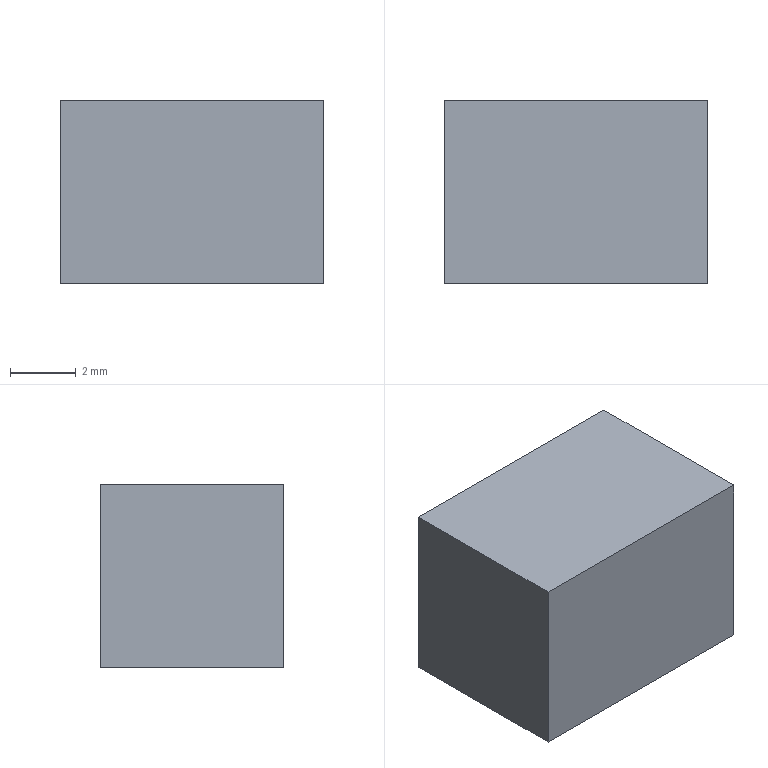Part | NX | features solid 2 | 1 solid | 6 faces | box 8 x 5.597 x 5.597 mm | volume 250.642 mm3 | plane 6
STEP:
#1=CARTESIAN_POINT('',(2258.,502.218,-669.685));
#2=VERTEX_POINT('',#1);
#3=CARTESIAN_POINT('',(2258.,507.815,-669.685));
#4=VERTEX_POINT('',#3);
#5=CARTESIAN_POINT('',(2258.,507.815,-669.685));
#6=DIRECTION('',(0.,1.,0.));
#7=VECTOR('',#6,1000.);
#8=LINE('',#5,#7);
#9=EDGE_CURVE('',#2,#4,#8,.T.);
#10=ORIENTED_EDGE('',*,*,#9,.F.);
#11=CARTESIAN_POINT('',(2250.,502.218,-669.685));
#12=VERTEX_POINT('',#11);
#13=CARTESIAN_POINT('',(2250.,502.218,-669.685));
#14=DIRECTION('',(1.,0.,0.));
#15=VECTOR('',#14,1000.);
#16=LINE('',#13,#15);
#17=EDGE_CURVE('',#12,#2,#16,.T.);
#18=ORIENTED_EDGE('',*,*,#17,.F.);
#19=CARTESIAN_POINT('',(2250.,507.815,-669.685));
#20=VERTEX_POINT('',#19);
#21=CARTESIAN_POINT('',(2250.,507.815,-669.685));
#22=CARTESIAN_POINT('',(2250.,505.949,-669.685));
#23=CARTESIAN_POINT('',(2250.,504.084,-669.685));
#24=CARTESIAN_POINT('',(2250.,502.218,-669.685));
#25=B_SPLINE_CURVE_WITH_KNOTS('',3,(#21,#22,#23,#24),.UNSPECIFIED.,.F.,.F.,(4,4),(0.,0.25),.PIECEWISE_BEZIER_KNOTS.);
#26=EDGE_CURVE('',#20,#12,#25,.T.);
#27=ORIENTED_EDGE('',*,*,#26,.F.);
#28=CARTESIAN_POINT('',(2250.,507.815,-669.685));
#29=DIRECTION('',(1.,0.,0.));
#30=VECTOR('',#29,1000.);
#31=LINE('',#28,#30);
#32=EDGE_CURVE('',#20,#4,#31,.T.);
#33=ORIENTED_EDGE('',*,*,#32,.T.);
#34=EDGE_LOOP('',(#10,#18,#27,#33));
#35=FACE_BOUND('',#34,.T.);
#36=CARTESIAN_POINT('',(2250.,507.815,-669.685));
#37=DIRECTION('',(0.,0.,-1.));
#38=DIRECTION('',(1.,0.,0.));
#39=AXIS2_PLACEMENT_3D('',#36,#37,#38);
#40=PLANE('',#39);
#41=ADVANCED_FACE('',(#35),#40,.T.);
#42=CARTESIAN_POINT('',(2258.,502.218,-664.088));
#43=VERTEX_POINT('',#42);
#44=CARTESIAN_POINT('',(2258.,502.218,-669.685));
#45=DIRECTION('',(0.,0.,-1.));
#46=VECTOR('',#45,1000.);
#47=LINE('',#44,#46);
#48=EDGE_CURVE('',#43,#2,#47,.T.);
#49=ORIENTED_EDGE('',*,*,#48,.F.);
#50=CARTESIAN_POINT('',(2250.,502.218,-664.088));
#51=VERTEX_POINT('',#50);
#52=CARTESIAN_POINT('',(2250.,502.218,-664.088));
#53=DIRECTION('',(1.,0.,0.));
#54=VECTOR('',#53,1000.);
#55=LINE('',#52,#54);
#56=EDGE_CURVE('',#51,#43,#55,.T.);
#57=ORIENTED_EDGE('',*,*,#56,.F.);
#58=CARTESIAN_POINT('',(2250.,502.218,-669.685));
#59=CARTESIAN_POINT('',(2250.,502.218,-667.82));
#60=CARTESIAN_POINT('',(2250.,502.218,-665.954));
#61=CARTESIAN_POINT('',(2250.,502.218,-664.088));
#62=B_SPLINE_CURVE_WITH_KNOTS('',3,(#58,#59,#60,#61),.UNSPECIFIED.,.F.,.F.,(4,4),(0.25,0.5),.PIECEWISE_BEZIER_KNOTS.);
#63=EDGE_CURVE('',#12,#51,#62,.T.);
#64=ORIENTED_EDGE('',*,*,#63,.F.);
#65=ORIENTED_EDGE('',*,*,#17,.T.);
#66=EDGE_LOOP('',(#49,#57,#64,#65));
#67=FACE_BOUND('',#66,.T.);
#68=CARTESIAN_POINT('',(2250.,502.218,-669.685));
#69=DIRECTION('',(0.,-1.,0.));
#70=DIRECTION('',(-1.,0.,0.));
#71=AXIS2_PLACEMENT_3D('',#68,#69,#70);
#72=PLANE('',#71);
#73=ADVANCED_FACE('',(#67),#72,.T.);
#74=CARTESIAN_POINT('',(2258.,507.815,-664.088));
#75=VERTEX_POINT('',#74);
#76=CARTESIAN_POINT('',(2258.,502.218,-664.088));
#77=DIRECTION('',(0.,-1.,0.));
#78=VECTOR('',#77,1000.);
#79=LINE('',#76,#78);
#80=EDGE_CURVE('',#75,#43,#79,.T.);
#81=ORIENTED_EDGE('',*,*,#80,.F.);
#82=CARTESIAN_POINT('',(2250.,507.815,-664.088));
#83=VERTEX_POINT('',#82);
#84=CARTESIAN_POINT('',(2250.,507.815,-664.088));
#85=DIRECTION('',(1.,0.,0.));
#86=VECTOR('',#85,1000.);
#87=LINE('',#84,#86);
#88=EDGE_CURVE('',#83,#75,#87,.T.);
#89=ORIENTED_EDGE('',*,*,#88,.F.);
#90=CARTESIAN_POINT('',(2250.,502.218,-664.088));
#91=CARTESIAN_POINT('',(2250.,504.084,-664.088));
#92=CARTESIAN_POINT('',(2250.,505.949,-664.088));
#93=CARTESIAN_POINT('',(2250.,507.815,-664.088));
#94=B_SPLINE_CURVE_WITH_KNOTS('',3,(#90,#91,#92,#93),.UNSPECIFIED.,.F.,.F.,(4,4),(0.5,0.75),.PIECEWISE_BEZIER_KNOTS.);
#95=EDGE_CURVE('',#51,#83,#94,.T.);
#96=ORIENTED_EDGE('',*,*,#95,.F.);
#97=ORIENTED_EDGE('',*,*,#56,.T.);
#98=EDGE_LOOP('',(#81,#89,#96,#97));
#99=FACE_BOUND('',#98,.T.);
#100=CARTESIAN_POINT('',(2250.,502.218,-664.088));
#101=DIRECTION('',(0.,0.,1.));
#102=DIRECTION('',(-1.,0.,0.));
#103=AXIS2_PLACEMENT_3D('',#100,#101,#102);
#104=PLANE('',#103);
#105=ADVANCED_FACE('',(#99),#104,.T.);
#106=CARTESIAN_POINT('',(2258.,507.815,-664.088));
#107=DIRECTION('',(0.,0.,1.));
#108=VECTOR('',#107,1000.);
#109=LINE('',#106,#108);
#110=EDGE_CURVE('',#4,#75,#109,.T.);
#111=ORIENTED_EDGE('',*,*,#110,.F.);
#112=ORIENTED_EDGE('',*,*,#32,.F.);
#113=CARTESIAN_POINT('',(2250.,507.815,-664.088));
#114=CARTESIAN_POINT('',(2250.,507.815,-665.954));
#115=CARTESIAN_POINT('',(2250.,507.815,-667.82));
#116=CARTESIAN_POINT('',(2250.,507.815,-669.685));
#117=B_SPLINE_CURVE_WITH_KNOTS('',3,(#113,#114,#115,#116),.UNSPECIFIED.,.F.,.F.,(4,4),(0.75,1.),.PIECEWISE_BEZIER_KNOTS.);
#118=EDGE_CURVE('',#83,#20,#117,.T.);
#119=ORIENTED_EDGE('',*,*,#118,.F.);
#120=ORIENTED_EDGE('',*,*,#88,.T.);
#121=EDGE_LOOP('',(#111,#112,#119,#120));
#122=FACE_BOUND('',#121,.T.);
#123=CARTESIAN_POINT('',(2250.,507.815,-664.088));
#124=DIRECTION('',(0.,1.,0.));
#125=DIRECTION('',(1.,0.,0.));
#126=AXIS2_PLACEMENT_3D('',#123,#124,#125);
#127=PLANE('',#126);
#128=ADVANCED_FACE('',(#122),#127,.T.);
#129=ORIENTED_EDGE('',*,*,#26,.T.);
#130=ORIENTED_EDGE('',*,*,#63,.T.);
#131=ORIENTED_EDGE('',*,*,#95,.T.);
#132=ORIENTED_EDGE('',*,*,#118,.T.);
#133=EDGE_LOOP('',(#129,#130,#131,#132));
#134=FACE_BOUND('',#133,.T.);
#135=CARTESIAN_POINT('',(2250.,505.017,-669.685));
#136=DIRECTION('',(-1.,0.,0.));
#137=DIRECTION('',(0.,1.,0.));
#138=AXIS2_PLACEMENT_3D('',#135,#136,#137);
#139=PLANE('',#138);
#140=ADVANCED_FACE('',(#134),#139,.T.);
#141=ORIENTED_EDGE('',*,*,#48,.T.);
#142=ORIENTED_EDGE('',*,*,#9,.T.);
#143=ORIENTED_EDGE('',*,*,#110,.T.);
#144=ORIENTED_EDGE('',*,*,#80,.T.);
#145=EDGE_LOOP('',(#141,#142,#143,#144));
#146=FACE_BOUND('',#145,.T.);
#147=CARTESIAN_POINT('',(2258.,483.819,-626.247));
#148=DIRECTION('',(-1.,0.,0.));
#149=DIRECTION('',(0.,0.,-1.));
#150=AXIS2_PLACEMENT_3D('',#147,#148,#149);
#151=PLANE('',#150);
#152=ADVANCED_FACE('',(#146),#151,.F.);
#153=CLOSED_SHELL('',(#41,#73,#105,#128,#140,#152));
#154=MANIFOLD_SOLID_BREP('',#153);
#155=(LENGTH_UNIT()NAMED_UNIT(*)SI_UNIT(.MILLI.,.METRE.));
#156=UNCERTAINTY_MEASURE_WITH_UNIT(LENGTH_MEASURE(0.00001),#155,'','');
#157=(NAMED_UNIT(*)PLANE_ANGLE_UNIT()SI_UNIT($,.RADIAN.));
#158=(NAMED_UNIT(*)SI_UNIT($,.STERADIAN.)SOLID_ANGLE_UNIT());
#159=(GEOMETRIC_REPRESENTATION_CONTEXT(3)GLOBAL_UNCERTAINTY_ASSIGNED_CONTEXT((#156))GLOBAL_UNIT_ASSIGNED_CONTEXT((#155,#157,#158))REPRESENTATION_CONTEXT('',''));
#160=ADVANCED_BREP_SHAPE_REPRESENTATION('',(#154),#159);